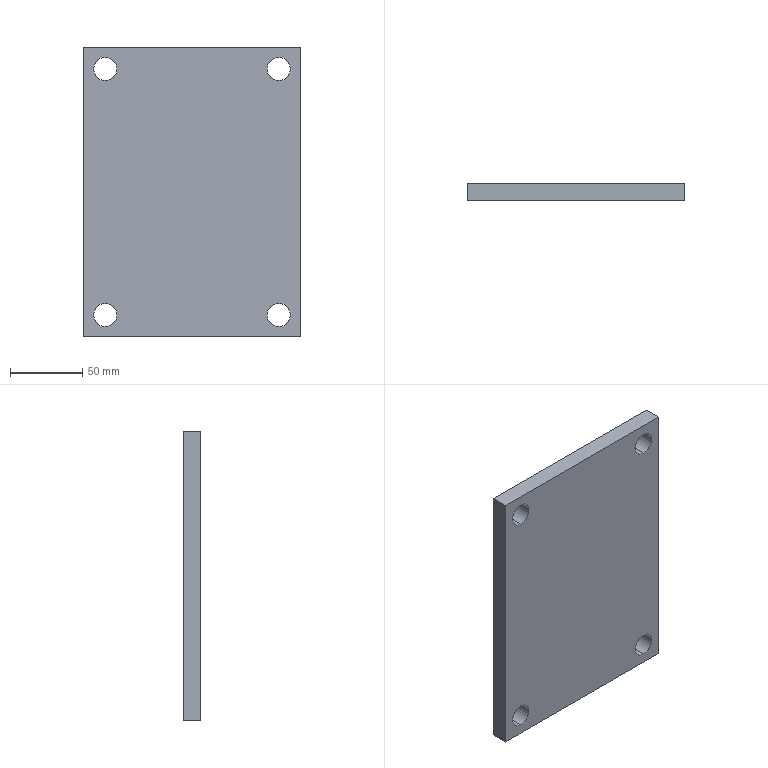Part | STEP file | E3-楼梯立柱Pad 1 | 1 solid | 14 faces | box 150 x 12 x 200 mm | volume 350349 mm3 | cylinder 8 | plane 6 | commonest cylinder face diameters 16 x8
STEP:
#1=CARTESIAN_POINT('',(0.,0.,0.));
#2=DIRECTION('',(0.,0.,1.));
#3=DIRECTION('',(1.,0.,0.));
#4=AXIS2_PLACEMENT_3D('',#1,#2,#3);
#5=CARTESIAN_POINT('',(60.,0.,-93.));
#6=VERTEX_POINT('',#5);
#7=CARTESIAN_POINT('',(60.,12.,-93.));
#8=VERTEX_POINT('',#7);
#9=CARTESIAN_POINT('',(60.,12.,-93.));
#10=DIRECTION('',(0.,1.,0.));
#11=VECTOR('',#10,1.);
#12=LINE('',#9,#11);
#13=CARTESIAN_POINT('',(60.,12.,-85.));
#14=DIRECTION('',(0.,1.,0.));
#15=DIRECTION('',(0.,0.,-1.));
#16=AXIS2_PLACEMENT_3D('',#13,#14,#15);
#17=CYLINDRICAL_SURFACE('',#16,8.);
#18=CARTESIAN_POINT('',(6.283,0.));
#19=DIRECTION('',(0.,1.));
#20=VECTOR('',#19,1.);
#21=LINE('',#18,#20);
#22=(GEOMETRIC_REPRESENTATION_CONTEXT(2)PARAMETRIC_REPRESENTATION_CONTEXT()REPRESENTATION_CONTEXT('',''));
#23=DEFINITIONAL_REPRESENTATION('',(#21),#22);
#24=PCURVE('',#17,#23);
#25=CARTESIAN_POINT('',(60.,12.,-85.));
#26=DIRECTION('',(0.,1.,0.));
#27=DIRECTION('',(0.,0.,-1.));
#28=AXIS2_PLACEMENT_3D('',#25,#26,#27);
#29=CYLINDRICAL_SURFACE('',#28,8.);
#30=CARTESIAN_POINT('',(0.,0.));
#31=DIRECTION('',(0.,1.));
#32=VECTOR('',#31,1.);
#33=LINE('',#30,#32);
#34=(GEOMETRIC_REPRESENTATION_CONTEXT(2)PARAMETRIC_REPRESENTATION_CONTEXT()REPRESENTATION_CONTEXT('',''));
#35=DEFINITIONAL_REPRESENTATION('',(#33),#34);
#36=PCURVE('',#29,#35);
#37=SURFACE_CURVE('',#12,(#24,#36),.PCURVE_S1.);
#38=EDGE_CURVE('',#6,#8,#37,.T.);
#39=ORIENTED_EDGE('',*,*,#38,.T.);
#40=CARTESIAN_POINT('',(60.,12.,-77.));
#41=VERTEX_POINT('',#40);
#42=CARTESIAN_POINT('',(60.,12.,-85.));
#43=DIRECTION('',(0.,-1.,0.));
#44=DIRECTION('',(0.,0.,-1.));
#45=AXIS2_PLACEMENT_3D('',#42,#43,#44);
#46=CIRCLE('',#45,8.);
#47=CARTESIAN_POINT('',(6.283,0.));
#48=DIRECTION('',(-1.,0.));
#49=VECTOR('',#48,1.);
#50=LINE('',#47,#49);
#51=(GEOMETRIC_REPRESENTATION_CONTEXT(2)PARAMETRIC_REPRESENTATION_CONTEXT()REPRESENTATION_CONTEXT('',''));
#52=DEFINITIONAL_REPRESENTATION('',(#50),#51);
#53=PCURVE('',#17,#52);
#54=CARTESIAN_POINT('',(0.,12.,0.));
#55=DIRECTION('',(0.,1.,0.));
#56=DIRECTION('',(0.,0.,-1.));
#57=AXIS2_PLACEMENT_3D('',#54,#55,#56);
#58=PLANE('',#57);
#59=CARTESIAN_POINT('',(93.,-60.));
#60=CARTESIAN_POINT('',(93.,-73.856));
#61=CARTESIAN_POINT('',(81.,-66.928));
#62=CARTESIAN_POINT('',(69.,-60.));
#63=CARTESIAN_POINT('',(81.,-53.072));
#64=CARTESIAN_POINT('',(93.,-46.144));
#65=CARTESIAN_POINT('',(93.,-60.));
#66=(BOUNDED_CURVE()B_SPLINE_CURVE(2,(#59,#60,#61,#62,#63,#64,#65),.UNSPECIFIED.,.T.,.F.)B_SPLINE_CURVE_WITH_KNOTS((1,2,2,2,2,1),(-2.094,0.,2.094,4.189,6.283,8.378),.UNSPECIFIED.)CURVE()GEOMETRIC_REPRESENTATION_ITEM()RATIONAL_B_SPLINE_CURVE((1.,0.5,1.,0.5,1.,0.5,1.))REPRESENTATION_ITEM(''));
#67=(GEOMETRIC_REPRESENTATION_CONTEXT(2)PARAMETRIC_REPRESENTATION_CONTEXT()REPRESENTATION_CONTEXT('',''));
#68=DEFINITIONAL_REPRESENTATION('',(#66),#67);
#69=PCURVE('',#58,#68);
#70=SURFACE_CURVE('',#46,(#53,#69),.PCURVE_S1.);
#71=EDGE_CURVE('',#8,#41,#70,.T.);
#72=ORIENTED_EDGE('',*,*,#71,.T.);
#73=CARTESIAN_POINT('',(60.,0.,-77.));
#74=VERTEX_POINT('',#73);
#75=CARTESIAN_POINT('',(60.,12.,-77.));
#76=DIRECTION('',(0.,1.,0.));
#77=VECTOR('',#76,1.);
#78=LINE('',#75,#77);
#79=CARTESIAN_POINT('',(3.142,0.));
#80=DIRECTION('',(0.,1.));
#81=VECTOR('',#80,1.);
#82=LINE('',#79,#81);
#83=(GEOMETRIC_REPRESENTATION_CONTEXT(2)PARAMETRIC_REPRESENTATION_CONTEXT()REPRESENTATION_CONTEXT('',''));
#84=DEFINITIONAL_REPRESENTATION('',(#82),#83);
#85=PCURVE('',#17,#84);
#86=CARTESIAN_POINT('',(3.142,0.));
#87=DIRECTION('',(0.,1.));
#88=VECTOR('',#87,1.);
#89=LINE('',#86,#88);
#90=(GEOMETRIC_REPRESENTATION_CONTEXT(2)PARAMETRIC_REPRESENTATION_CONTEXT()REPRESENTATION_CONTEXT('',''));
#91=DEFINITIONAL_REPRESENTATION('',(#89),#90);
#92=PCURVE('',#29,#91);
#93=SURFACE_CURVE('',#78,(#85,#92),.PCURVE_S1.);
#94=EDGE_CURVE('',#74,#41,#93,.T.);
#95=ORIENTED_EDGE('',*,*,#94,.F.);
#96=CARTESIAN_POINT('',(60.,0.,-85.));
#97=DIRECTION('',(0.,-1.,0.));
#98=DIRECTION('',(0.,0.,-1.));
#99=AXIS2_PLACEMENT_3D('',#96,#97,#98);
#100=CIRCLE('',#99,8.);
#101=CARTESIAN_POINT('',(6.283,-12.));
#102=DIRECTION('',(-1.,0.));
#103=VECTOR('',#102,1.);
#104=LINE('',#101,#103);
#105=(GEOMETRIC_REPRESENTATION_CONTEXT(2)PARAMETRIC_REPRESENTATION_CONTEXT()REPRESENTATION_CONTEXT('',''));
#106=DEFINITIONAL_REPRESENTATION('',(#104),#105);
#107=PCURVE('',#17,#106);
#108=CARTESIAN_POINT('',(0.,0.,0.));
#109=DIRECTION('',(0.,1.,0.));
#110=DIRECTION('',(0.,0.,-1.));
#111=AXIS2_PLACEMENT_3D('',#108,#109,#110);
#112=PLANE('',#111);
#113=CARTESIAN_POINT('',(93.,-60.));
#114=CARTESIAN_POINT('',(93.,-73.856));
#115=CARTESIAN_POINT('',(81.,-66.928));
#116=CARTESIAN_POINT('',(69.,-60.));
#117=CARTESIAN_POINT('',(81.,-53.072));
#118=CARTESIAN_POINT('',(93.,-46.144));
#119=CARTESIAN_POINT('',(93.,-60.));
#120=(BOUNDED_CURVE()B_SPLINE_CURVE(2,(#113,#114,#115,#116,#117,#118,#119),.UNSPECIFIED.,.T.,.F.)B_SPLINE_CURVE_WITH_KNOTS((1,2,2,2,2,1),(-2.094,0.,2.094,4.189,6.283,8.378),.UNSPECIFIED.)CURVE()GEOMETRIC_REPRESENTATION_ITEM()RATIONAL_B_SPLINE_CURVE((1.,0.5,1.,0.5,1.,0.5,1.))REPRESENTATION_ITEM(''));
#121=(GEOMETRIC_REPRESENTATION_CONTEXT(2)PARAMETRIC_REPRESENTATION_CONTEXT()REPRESENTATION_CONTEXT('',''));
#122=DEFINITIONAL_REPRESENTATION('',(#120),#121);
#123=PCURVE('',#112,#122);
#124=SURFACE_CURVE('',#100,(#107,#123),.PCURVE_S1.);
#125=EDGE_CURVE('',#6,#74,#124,.T.);
#126=ORIENTED_EDGE('',*,*,#125,.F.);
#127=EDGE_LOOP('',(#39,#72,#95,#126));
#128=FACE_BOUND('',#127,.F.);
#129=ADVANCED_FACE('',(#128),#17,.F.);
#130=CARTESIAN_POINT('',(-60.,0.,77.));
#131=VERTEX_POINT('',#130);
#132=CARTESIAN_POINT('',(-60.,12.,77.));
#133=VERTEX_POINT('',#132);
#134=CARTESIAN_POINT('',(-60.,12.,77.));
#135=DIRECTION('',(0.,1.,0.));
#136=VECTOR('',#135,1.);
#137=LINE('',#134,#136);
#138=CARTESIAN_POINT('',(-60.,12.,85.));
#139=DIRECTION('',(0.,1.,0.));
#140=DIRECTION('',(0.,0.,-1.));
#141=AXIS2_PLACEMENT_3D('',#138,#139,#140);
#142=CYLINDRICAL_SURFACE('',#141,8.);
#143=CARTESIAN_POINT('',(6.283,0.));
#144=DIRECTION('',(0.,1.));
#145=VECTOR('',#144,1.);
#146=LINE('',#143,#145);
#147=(GEOMETRIC_REPRESENTATION_CONTEXT(2)PARAMETRIC_REPRESENTATION_CONTEXT()REPRESENTATION_CONTEXT('',''));
#148=DEFINITIONAL_REPRESENTATION('',(#146),#147);
#149=PCURVE('',#142,#148);
#150=CARTESIAN_POINT('',(-60.,12.,85.));
#151=DIRECTION('',(0.,1.,0.));
#152=DIRECTION('',(0.,0.,-1.));
#153=AXIS2_PLACEMENT_3D('',#150,#151,#152);
#154=CYLINDRICAL_SURFACE('',#153,8.);
#155=CARTESIAN_POINT('',(0.,0.));
#156=DIRECTION('',(0.,1.));
#157=VECTOR('',#156,1.);
#158=LINE('',#155,#157);
#159=(GEOMETRIC_REPRESENTATION_CONTEXT(2)PARAMETRIC_REPRESENTATION_CONTEXT()REPRESENTATION_CONTEXT('',''));
#160=DEFINITIONAL_REPRESENTATION('',(#158),#159);
#161=PCURVE('',#154,#160);
#162=SURFACE_CURVE('',#137,(#149,#161),.PCURVE_S1.);
#163=EDGE_CURVE('',#131,#133,#162,.T.);
#164=ORIENTED_EDGE('',*,*,#163,.T.);
#165=CARTESIAN_POINT('',(-60.,12.,93.));
#166=VERTEX_POINT('',#165);
#167=CARTESIAN_POINT('',(-60.,12.,85.));
#168=DIRECTION('',(0.,-1.,0.));
#169=DIRECTION('',(0.,0.,-1.));
#170=AXIS2_PLACEMENT_3D('',#167,#168,#169);
#171=CIRCLE('',#170,8.);
#172=CARTESIAN_POINT('',(6.283,0.));
#173=DIRECTION('',(-1.,0.));
#174=VECTOR('',#173,1.);
#175=LINE('',#172,#174);
#176=(GEOMETRIC_REPRESENTATION_CONTEXT(2)PARAMETRIC_REPRESENTATION_CONTEXT()REPRESENTATION_CONTEXT('',''));
#177=DEFINITIONAL_REPRESENTATION('',(#175),#176);
#178=PCURVE('',#142,#177);
#179=CARTESIAN_POINT('',(-77.,60.));
#180=CARTESIAN_POINT('',(-77.,46.144));
#181=CARTESIAN_POINT('',(-89.,53.072));
#182=CARTESIAN_POINT('',(-101.,60.));
#183=CARTESIAN_POINT('',(-89.,66.928));
#184=CARTESIAN_POINT('',(-77.,73.856));
#185=CARTESIAN_POINT('',(-77.,60.));
#186=(BOUNDED_CURVE()B_SPLINE_CURVE(2,(#179,#180,#181,#182,#183,#184,#185),.UNSPECIFIED.,.T.,.F.)B_SPLINE_CURVE_WITH_KNOTS((1,2,2,2,2,1),(-2.094,0.,2.094,4.189,6.283,8.378),.UNSPECIFIED.)CURVE()GEOMETRIC_REPRESENTATION_ITEM()RATIONAL_B_SPLINE_CURVE((1.,0.5,1.,0.5,1.,0.5,1.))REPRESENTATION_ITEM(''));
#187=(GEOMETRIC_REPRESENTATION_CONTEXT(2)PARAMETRIC_REPRESENTATION_CONTEXT()REPRESENTATION_CONTEXT('',''));
#188=DEFINITIONAL_REPRESENTATION('',(#186),#187);
#189=PCURVE('',#58,#188);
#190=SURFACE_CURVE('',#171,(#178,#189),.PCURVE_S1.);
#191=EDGE_CURVE('',#133,#166,#190,.T.);
#192=ORIENTED_EDGE('',*,*,#191,.T.);
#193=CARTESIAN_POINT('',(-60.,0.,93.));
#194=VERTEX_POINT('',#193);
#195=CARTESIAN_POINT('',(-60.,12.,93.));
#196=DIRECTION('',(0.,1.,0.));
#197=VECTOR('',#196,1.);
#198=LINE('',#195,#197);
#199=CARTESIAN_POINT('',(3.142,0.));
#200=DIRECTION('',(0.,1.));
#201=VECTOR('',#200,1.);
#202=LINE('',#199,#201);
#203=(GEOMETRIC_REPRESENTATION_CONTEXT(2)PARAMETRIC_REPRESENTATION_CONTEXT()REPRESENTATION_CONTEXT('',''));
#204=DEFINITIONAL_REPRESENTATION('',(#202),#203);
#205=PCURVE('',#142,#204);
#206=CARTESIAN_POINT('',(3.142,0.));
#207=DIRECTION('',(0.,1.));
#208=VECTOR('',#207,1.);
#209=LINE('',#206,#208);
#210=(GEOMETRIC_REPRESENTATION_CONTEXT(2)PARAMETRIC_REPRESENTATION_CONTEXT()REPRESENTATION_CONTEXT('',''));
#211=DEFINITIONAL_REPRESENTATION('',(#209),#210);
#212=PCURVE('',#154,#211);
#213=SURFACE_CURVE('',#198,(#205,#212),.PCURVE_S1.);
#214=EDGE_CURVE('',#194,#166,#213,.T.);
#215=ORIENTED_EDGE('',*,*,#214,.F.);
#216=CARTESIAN_POINT('',(-60.,0.,85.));
#217=DIRECTION('',(0.,-1.,0.));
#218=DIRECTION('',(0.,0.,-1.));
#219=AXIS2_PLACEMENT_3D('',#216,#217,#218);
#220=CIRCLE('',#219,8.);
#221=CARTESIAN_POINT('',(6.283,-12.));
#222=DIRECTION('',(-1.,0.));
#223=VECTOR('',#222,1.);
#224=LINE('',#221,#223);
#225=(GEOMETRIC_REPRESENTATION_CONTEXT(2)PARAMETRIC_REPRESENTATION_CONTEXT()REPRESENTATION_CONTEXT('',''));
#226=DEFINITIONAL_REPRESENTATION('',(#224),#225);
#227=PCURVE('',#142,#226);
#228=CARTESIAN_POINT('',(-77.,60.));
#229=CARTESIAN_POINT('',(-77.,46.144));
#230=CARTESIAN_POINT('',(-89.,53.072));
#231=CARTESIAN_POINT('',(-101.,60.));
#232=CARTESIAN_POINT('',(-89.,66.928));
#233=CARTESIAN_POINT('',(-77.,73.856));
#234=CARTESIAN_POINT('',(-77.,60.));
#235=(BOUNDED_CURVE()B_SPLINE_CURVE(2,(#228,#229,#230,#231,#232,#233,#234),.UNSPECIFIED.,.T.,.F.)B_SPLINE_CURVE_WITH_KNOTS((1,2,2,2,2,1),(-2.094,0.,2.094,4.189,6.283,8.378),.UNSPECIFIED.)CURVE()GEOMETRIC_REPRESENTATION_ITEM()RATIONAL_B_SPLINE_CURVE((1.,0.5,1.,0.5,1.,0.5,1.))REPRESENTATION_ITEM(''));
#236=(GEOMETRIC_REPRESENTATION_CONTEXT(2)PARAMETRIC_REPRESENTATION_CONTEXT()REPRESENTATION_CONTEXT('',''));
#237=DEFINITIONAL_REPRESENTATION('',(#235),#236);
#238=PCURVE('',#112,#237);
#239=SURFACE_CURVE('',#220,(#227,#238),.PCURVE_S1.);
#240=EDGE_CURVE('',#131,#194,#239,.T.);
#241=ORIENTED_EDGE('',*,*,#240,.F.);
#242=EDGE_LOOP('',(#164,#192,#215,#241));
#243=FACE_BOUND('',#242,.F.);
#244=ADVANCED_FACE('',(#243),#142,.F.);
#245=CARTESIAN_POINT('',(-60.,0.,-93.));
#246=VERTEX_POINT('',#245);
#247=CARTESIAN_POINT('',(-60.,12.,-93.));
#248=VERTEX_POINT('',#247);
#249=CARTESIAN_POINT('',(-60.,12.,-93.));
#250=DIRECTION('',(0.,1.,0.));
#251=VECTOR('',#250,1.);
#252=LINE('',#249,#251);
#253=CARTESIAN_POINT('',(-60.,12.,-85.));
#254=DIRECTION('',(0.,1.,0.));
#255=DIRECTION('',(0.,0.,-1.));
#256=AXIS2_PLACEMENT_3D('',#253,#254,#255);
#257=CYLINDRICAL_SURFACE('',#256,8.);
#258=CARTESIAN_POINT('',(6.283,0.));
#259=DIRECTION('',(0.,1.));
#260=VECTOR('',#259,1.);
#261=LINE('',#258,#260);
#262=(GEOMETRIC_REPRESENTATION_CONTEXT(2)PARAMETRIC_REPRESENTATION_CONTEXT()REPRESENTATION_CONTEXT('',''));
#263=DEFINITIONAL_REPRESENTATION('',(#261),#262);
#264=PCURVE('',#257,#263);
#265=CARTESIAN_POINT('',(-60.,12.,-85.));
#266=DIRECTION('',(0.,1.,0.));
#267=DIRECTION('',(0.,0.,-1.));
#268=AXIS2_PLACEMENT_3D('',#265,#266,#267);
#269=CYLINDRICAL_SURFACE('',#268,8.);
#270=CARTESIAN_POINT('',(0.,0.));
#271=DIRECTION('',(0.,1.));
#272=VECTOR('',#271,1.);
#273=LINE('',#270,#272);
#274=(GEOMETRIC_REPRESENTATION_CONTEXT(2)PARAMETRIC_REPRESENTATION_CONTEXT()REPRESENTATION_CONTEXT('',''));
#275=DEFINITIONAL_REPRESENTATION('',(#273),#274);
#276=PCURVE('',#269,#275);
#277=SURFACE_CURVE('',#252,(#264,#276),.PCURVE_S1.);
#278=EDGE_CURVE('',#246,#248,#277,.T.);
#279=ORIENTED_EDGE('',*,*,#278,.T.);
#280=CARTESIAN_POINT('',(-60.,12.,-77.));
#281=VERTEX_POINT('',#280);
#282=CARTESIAN_POINT('',(-60.,12.,-85.));
#283=DIRECTION('',(0.,-1.,0.));
#284=DIRECTION('',(0.,0.,-1.));
#285=AXIS2_PLACEMENT_3D('',#282,#283,#284);
#286=CIRCLE('',#285,8.);
#287=CARTESIAN_POINT('',(6.283,0.));
#288=DIRECTION('',(-1.,0.));
#289=VECTOR('',#288,1.);
#290=LINE('',#287,#289);
#291=(GEOMETRIC_REPRESENTATION_CONTEXT(2)PARAMETRIC_REPRESENTATION_CONTEXT()REPRESENTATION_CONTEXT('',''));
#292=DEFINITIONAL_REPRESENTATION('',(#290),#291);
#293=PCURVE('',#257,#292);
#294=CARTESIAN_POINT('',(93.,60.));
#295=CARTESIAN_POINT('',(93.,46.144));
#296=CARTESIAN_POINT('',(81.,53.072));
#297=CARTESIAN_POINT('',(69.,60.));
#298=CARTESIAN_POINT('',(81.,66.928));
#299=CARTESIAN_POINT('',(93.,73.856));
#300=CARTESIAN_POINT('',(93.,60.));
#301=(BOUNDED_CURVE()B_SPLINE_CURVE(2,(#294,#295,#296,#297,#298,#299,#300),.UNSPECIFIED.,.T.,.F.)B_SPLINE_CURVE_WITH_KNOTS((1,2,2,2,2,1),(-2.094,0.,2.094,4.189,6.283,8.378),.UNSPECIFIED.)CURVE()GEOMETRIC_REPRESENTATION_ITEM()RATIONAL_B_SPLINE_CURVE((1.,0.5,1.,0.5,1.,0.5,1.))REPRESENTATION_ITEM(''));
#302=(GEOMETRIC_REPRESENTATION_CONTEXT(2)PARAMETRIC_REPRESENTATION_CONTEXT()REPRESENTATION_CONTEXT('',''));
#303=DEFINITIONAL_REPRESENTATION('',(#301),#302);
#304=PCURVE('',#58,#303);
#305=SURFACE_CURVE('',#286,(#293,#304),.PCURVE_S1.);
#306=EDGE_CURVE('',#248,#281,#305,.T.);
#307=ORIENTED_EDGE('',*,*,#306,.T.);
#308=CARTESIAN_POINT('',(-60.,0.,-77.));
#309=VERTEX_POINT('',#308);
#310=CARTESIAN_POINT('',(-60.,12.,-77.));
#311=DIRECTION('',(0.,1.,0.));
#312=VECTOR('',#311,1.);
#313=LINE('',#310,#312);
#314=CARTESIAN_POINT('',(3.142,0.));
#315=DIRECTION('',(0.,1.));
#316=VECTOR('',#315,1.);
#317=LINE('',#314,#316);
#318=(GEOMETRIC_REPRESENTATION_CONTEXT(2)PARAMETRIC_REPRESENTATION_CONTEXT()REPRESENTATION_CONTEXT('',''));
#319=DEFINITIONAL_REPRESENTATION('',(#317),#318);
#320=PCURVE('',#257,#319);
#321=CARTESIAN_POINT('',(3.142,0.));
#322=DIRECTION('',(0.,1.));
#323=VECTOR('',#322,1.);
#324=LINE('',#321,#323);
#325=(GEOMETRIC_REPRESENTATION_CONTEXT(2)PARAMETRIC_REPRESENTATION_CONTEXT()REPRESENTATION_CONTEXT('',''));
#326=DEFINITIONAL_REPRESENTATION('',(#324),#325);
#327=PCURVE('',#269,#326);
#328=SURFACE_CURVE('',#313,(#320,#327),.PCURVE_S1.);
#329=EDGE_CURVE('',#309,#281,#328,.T.);
#330=ORIENTED_EDGE('',*,*,#329,.F.);
#331=CARTESIAN_POINT('',(-60.,0.,-85.));
#332=DIRECTION('',(0.,-1.,0.));
#333=DIRECTION('',(0.,0.,-1.));
#334=AXIS2_PLACEMENT_3D('',#331,#332,#333);
#335=CIRCLE('',#334,8.);
#336=CARTESIAN_POINT('',(6.283,-12.));
#337=DIRECTION('',(-1.,0.));
#338=VECTOR('',#337,1.);
#339=LINE('',#336,#338);
#340=(GEOMETRIC_REPRESENTATION_CONTEXT(2)PARAMETRIC_REPRESENTATION_CONTEXT()REPRESENTATION_CONTEXT('',''));
#341=DEFINITIONAL_REPRESENTATION('',(#339),#340);
#342=PCURVE('',#257,#341);
#343=CARTESIAN_POINT('',(93.,60.));
#344=CARTESIAN_POINT('',(93.,46.144));
#345=CARTESIAN_POINT('',(81.,53.072));
#346=CARTESIAN_POINT('',(69.,60.));
#347=CARTESIAN_POINT('',(81.,66.928));
#348=CARTESIAN_POINT('',(93.,73.856));
#349=CARTESIAN_POINT('',(93.,60.));
#350=(BOUNDED_CURVE()B_SPLINE_CURVE(2,(#343,#344,#345,#346,#347,#348,#349),.UNSPECIFIED.,.T.,.F.)B_SPLINE_CURVE_WITH_KNOTS((1,2,2,2,2,1),(-2.094,0.,2.094,4.189,6.283,8.378),.UNSPECIFIED.)CURVE()GEOMETRIC_REPRESENTATION_ITEM()RATIONAL_B_SPLINE_CURVE((1.,0.5,1.,0.5,1.,0.5,1.))REPRESENTATION_ITEM(''));
#351=(GEOMETRIC_REPRESENTATION_CONTEXT(2)PARAMETRIC_REPRESENTATION_CONTEXT()REPRESENTATION_CONTEXT('',''));
#352=DEFINITIONAL_REPRESENTATION('',(#350),#351);
#353=PCURVE('',#112,#352);
#354=SURFACE_CURVE('',#335,(#342,#353),.PCURVE_S1.);
#355=EDGE_CURVE('',#246,#309,#354,.T.);
#356=ORIENTED_EDGE('',*,*,#355,.F.);
#357=EDGE_LOOP('',(#279,#307,#330,#356));
#358=FACE_BOUND('',#357,.F.);
#359=ADVANCED_FACE('',(#358),#257,.F.);
#360=CARTESIAN_POINT('',(60.,0.,77.));
#361=VERTEX_POINT('',#360);
#362=CARTESIAN_POINT('',(60.,12.,77.));
#363=VERTEX_POINT('',#362);
#364=CARTESIAN_POINT('',(60.,12.,77.));
#365=DIRECTION('',(0.,1.,0.));
#366=VECTOR('',#365,1.);
#367=LINE('',#364,#366);
#368=CARTESIAN_POINT('',(60.,12.,85.));
#369=DIRECTION('',(0.,1.,0.));
#370=DIRECTION('',(0.,0.,-1.));
#371=AXIS2_PLACEMENT_3D('',#368,#369,#370);
#372=CYLINDRICAL_SURFACE('',#371,8.);
#373=CARTESIAN_POINT('',(6.283,0.));
#374=DIRECTION('',(0.,1.));
#375=VECTOR('',#374,1.);
#376=LINE('',#373,#375);
#377=(GEOMETRIC_REPRESENTATION_CONTEXT(2)PARAMETRIC_REPRESENTATION_CONTEXT()REPRESENTATION_CONTEXT('',''));
#378=DEFINITIONAL_REPRESENTATION('',(#376),#377);
#379=PCURVE('',#372,#378);
#380=CARTESIAN_POINT('',(60.,12.,85.));
#381=DIRECTION('',(0.,1.,0.));
#382=DIRECTION('',(0.,0.,-1.));
#383=AXIS2_PLACEMENT_3D('',#380,#381,#382);
#384=CYLINDRICAL_SURFACE('',#383,8.);
#385=CARTESIAN_POINT('',(0.,0.));
#386=DIRECTION('',(0.,1.));
#387=VECTOR('',#386,1.);
#388=LINE('',#385,#387);
#389=(GEOMETRIC_REPRESENTATION_CONTEXT(2)PARAMETRIC_REPRESENTATION_CONTEXT()REPRESENTATION_CONTEXT('',''));
#390=DEFINITIONAL_REPRESENTATION('',(#388),#389);
#391=PCURVE('',#384,#390);
#392=SURFACE_CURVE('',#367,(#379,#391),.PCURVE_S1.);
#393=EDGE_CURVE('',#361,#363,#392,.T.);
#394=ORIENTED_EDGE('',*,*,#393,.T.);
#395=CARTESIAN_POINT('',(60.,12.,93.));
#396=VERTEX_POINT('',#395);
#397=CARTESIAN_POINT('',(60.,12.,85.));
#398=DIRECTION('',(0.,-1.,0.));
#399=DIRECTION('',(0.,0.,-1.));
#400=AXIS2_PLACEMENT_3D('',#397,#398,#399);
#401=CIRCLE('',#400,8.);
#402=CARTESIAN_POINT('',(6.283,0.));
#403=DIRECTION('',(-1.,0.));
#404=VECTOR('',#403,1.);
#405=LINE('',#402,#404);
#406=(GEOMETRIC_REPRESENTATION_CONTEXT(2)PARAMETRIC_REPRESENTATION_CONTEXT()REPRESENTATION_CONTEXT('',''));
#407=DEFINITIONAL_REPRESENTATION('',(#405),#406);
#408=PCURVE('',#372,#407);
#409=CARTESIAN_POINT('',(-77.,-60.));
#410=CARTESIAN_POINT('',(-77.,-73.856));
#411=CARTESIAN_POINT('',(-89.,-66.928));
#412=CARTESIAN_POINT('',(-101.,-60.));
#413=CARTESIAN_POINT('',(-89.,-53.072));
#414=CARTESIAN_POINT('',(-77.,-46.144));
#415=CARTESIAN_POINT('',(-77.,-60.));
#416=(BOUNDED_CURVE()B_SPLINE_CURVE(2,(#409,#410,#411,#412,#413,#414,#415),.UNSPECIFIED.,.T.,.F.)B_SPLINE_CURVE_WITH_KNOTS((1,2,2,2,2,1),(-2.094,0.,2.094,4.189,6.283,8.378),.UNSPECIFIED.)CURVE()GEOMETRIC_REPRESENTATION_ITEM()RATIONAL_B_SPLINE_CURVE((1.,0.5,1.,0.5,1.,0.5,1.))REPRESENTATION_ITEM(''));
#417=(GEOMETRIC_REPRESENTATION_CONTEXT(2)PARAMETRIC_REPRESENTATION_CONTEXT()REPRESENTATION_CONTEXT('',''));
#418=DEFINITIONAL_REPRESENTATION('',(#416),#417);
#419=PCURVE('',#58,#418);
#420=SURFACE_CURVE('',#401,(#408,#419),.PCURVE_S1.);
#421=EDGE_CURVE('',#363,#396,#420,.T.);
#422=ORIENTED_EDGE('',*,*,#421,.T.);
#423=CARTESIAN_POINT('',(60.,0.,93.));
#424=VERTEX_POINT('',#423);
#425=CARTESIAN_POINT('',(60.,12.,93.));
#426=DIRECTION('',(0.,1.,0.));
#427=VECTOR('',#426,1.);
#428=LINE('',#425,#427);
#429=CARTESIAN_POINT('',(3.142,0.));
#430=DIRECTION('',(0.,1.));
#431=VECTOR('',#430,1.);
#432=LINE('',#429,#431);
#433=(GEOMETRIC_REPRESENTATION_CONTEXT(2)PARAMETRIC_REPRESENTATION_CONTEXT()REPRESENTATION_CONTEXT('',''));
#434=DEFINITIONAL_REPRESENTATION('',(#432),#433);
#435=PCURVE('',#372,#434);
#436=CARTESIAN_POINT('',(3.142,0.));
#437=DIRECTION('',(0.,1.));
#438=VECTOR('',#437,1.);
#439=LINE('',#436,#438);
#440=(GEOMETRIC_REPRESENTATION_CONTEXT(2)PARAMETRIC_REPRESENTATION_CONTEXT()REPRESENTATION_CONTEXT('',''));
#441=DEFINITIONAL_REPRESENTATION('',(#439),#440);
#442=PCURVE('',#384,#441);
#443=SURFACE_CURVE('',#428,(#435,#442),.PCURVE_S1.);
#444=EDGE_CURVE('',#424,#396,#443,.T.);
#445=ORIENTED_EDGE('',*,*,#444,.F.);
#446=CARTESIAN_POINT('',(60.,0.,85.));
#447=DIRECTION('',(0.,-1.,0.));
#448=DIRECTION('',(0.,0.,-1.));
#449=AXIS2_PLACEMENT_3D('',#446,#447,#448);
#450=CIRCLE('',#449,8.);
#451=CARTESIAN_POINT('',(6.283,-12.));
#452=DIRECTION('',(-1.,0.));
#453=VECTOR('',#452,1.);
#454=LINE('',#451,#453);
#455=(GEOMETRIC_REPRESENTATION_CONTEXT(2)PARAMETRIC_REPRESENTATION_CONTEXT()REPRESENTATION_CONTEXT('',''));
#456=DEFINITIONAL_REPRESENTATION('',(#454),#455);
#457=PCURVE('',#372,#456);
#458=CARTESIAN_POINT('',(-77.,-60.));
#459=CARTESIAN_POINT('',(-77.,-73.856));
#460=CARTESIAN_POINT('',(-89.,-66.928));
#461=CARTESIAN_POINT('',(-101.,-60.));
#462=CARTESIAN_POINT('',(-89.,-53.072));
#463=CARTESIAN_POINT('',(-77.,-46.144));
#464=CARTESIAN_POINT('',(-77.,-60.));
#465=(BOUNDED_CURVE()B_SPLINE_CURVE(2,(#458,#459,#460,#461,#462,#463,#464),.UNSPECIFIED.,.T.,.F.)B_SPLINE_CURVE_WITH_KNOTS((1,2,2,2,2,1),(-2.094,0.,2.094,4.189,6.283,8.378),.UNSPECIFIED.)CURVE()GEOMETRIC_REPRESENTATION_ITEM()RATIONAL_B_SPLINE_CURVE((1.,0.5,1.,0.5,1.,0.5,1.))REPRESENTATION_ITEM(''));
#466=(GEOMETRIC_REPRESENTATION_CONTEXT(2)PARAMETRIC_REPRESENTATION_CONTEXT()REPRESENTATION_CONTEXT('',''));
#467=DEFINITIONAL_REPRESENTATION('',(#465),#466);
#468=PCURVE('',#112,#467);
#469=SURFACE_CURVE('',#450,(#457,#468),.PCURVE_S1.);
#470=EDGE_CURVE('',#361,#424,#469,.T.);
#471=ORIENTED_EDGE('',*,*,#470,.F.);
#472=EDGE_LOOP('',(#394,#422,#445,#471));
#473=FACE_BOUND('',#472,.F.);
#474=ADVANCED_FACE('',(#473),#372,.F.);
#475=CARTESIAN_POINT('',(75.,0.,-100.));
#476=VERTEX_POINT('',#475);
#477=CARTESIAN_POINT('',(75.,0.,100.));
#478=VERTEX_POINT('',#477);
#479=CARTESIAN_POINT('',(75.,0.,100.));
#480=DIRECTION('',(0.,0.,1.));
#481=VECTOR('',#480,1.);
#482=LINE('',#479,#481);
#483=CARTESIAN_POINT('',(75.,12.,100.));
#484=DIRECTION('',(-1.,0.,0.));
#485=DIRECTION('',(0.,0.,-1.));
#486=AXIS2_PLACEMENT_3D('',#483,#484,#485);
#487=PLANE('',#486);
#488=CARTESIAN_POINT('',(0.,12.));
#489=DIRECTION('',(-1.,0.));
#490=VECTOR('',#489,1.);
#491=LINE('',#488,#490);
#492=(GEOMETRIC_REPRESENTATION_CONTEXT(2)PARAMETRIC_REPRESENTATION_CONTEXT()REPRESENTATION_CONTEXT('',''));
#493=DEFINITIONAL_REPRESENTATION('',(#491),#492);
#494=PCURVE('',#487,#493);
#495=CARTESIAN_POINT('',(-100.,-75.));
#496=DIRECTION('',(-1.,0.));
#497=VECTOR('',#496,1.);
#498=LINE('',#495,#497);
#499=(GEOMETRIC_REPRESENTATION_CONTEXT(2)PARAMETRIC_REPRESENTATION_CONTEXT()REPRESENTATION_CONTEXT('',''));
#500=DEFINITIONAL_REPRESENTATION('',(#498),#499);
#501=PCURVE('',#112,#500);
#502=SURFACE_CURVE('',#482,(#494,#501),.PCURVE_S1.);
#503=EDGE_CURVE('',#476,#478,#502,.T.);
#504=ORIENTED_EDGE('',*,*,#503,.F.);
#505=CARTESIAN_POINT('',(75.,12.,-100.));
#506=VERTEX_POINT('',#505);
#507=CARTESIAN_POINT('',(75.,12.,-100.));
#508=DIRECTION('',(0.,-1.,0.));
#509=VECTOR('',#508,1.);
#510=LINE('',#507,#509);
#511=CARTESIAN_POINT('',(200.,0.));
#512=DIRECTION('',(0.,1.));
#513=VECTOR('',#512,1.);
#514=LINE('',#511,#513);
#515=(GEOMETRIC_REPRESENTATION_CONTEXT(2)PARAMETRIC_REPRESENTATION_CONTEXT()REPRESENTATION_CONTEXT('',''));
#516=DEFINITIONAL_REPRESENTATION('',(#514),#515);
#517=PCURVE('',#487,#516);
#518=CARTESIAN_POINT('',(-75.,12.,-100.));
#519=DIRECTION('',(0.,0.,1.));
#520=DIRECTION('',(-1.,0.,0.));
#521=AXIS2_PLACEMENT_3D('',#518,#519,#520);
#522=PLANE('',#521);
#523=CARTESIAN_POINT('',(-150.,0.));
#524=DIRECTION('',(0.,1.));
#525=VECTOR('',#524,1.);
#526=LINE('',#523,#525);
#527=(GEOMETRIC_REPRESENTATION_CONTEXT(2)PARAMETRIC_REPRESENTATION_CONTEXT()REPRESENTATION_CONTEXT('',''));
#528=DEFINITIONAL_REPRESENTATION('',(#526),#527);
#529=PCURVE('',#522,#528);
#530=SURFACE_CURVE('',#510,(#517,#529),.PCURVE_S1.);
#531=EDGE_CURVE('',#506,#476,#530,.T.);
#532=ORIENTED_EDGE('',*,*,#531,.F.);
#533=CARTESIAN_POINT('',(75.,12.,100.));
#534=VERTEX_POINT('',#533);
#535=CARTESIAN_POINT('',(75.,12.,100.));
#536=DIRECTION('',(0.,0.,1.));
#537=VECTOR('',#536,1.);
#538=LINE('',#535,#537);
#539=CARTESIAN_POINT('',(0.,0.));
#540=DIRECTION('',(-1.,0.));
#541=VECTOR('',#540,1.);
#542=LINE('',#539,#541);
#543=(GEOMETRIC_REPRESENTATION_CONTEXT(2)PARAMETRIC_REPRESENTATION_CONTEXT()REPRESENTATION_CONTEXT('',''));
#544=DEFINITIONAL_REPRESENTATION('',(#542),#543);
#545=PCURVE('',#487,#544);
#546=CARTESIAN_POINT('',(-100.,-75.));
#547=DIRECTION('',(-1.,0.));
#548=VECTOR('',#547,1.);
#549=LINE('',#546,#548);
#550=(GEOMETRIC_REPRESENTATION_CONTEXT(2)PARAMETRIC_REPRESENTATION_CONTEXT()REPRESENTATION_CONTEXT('',''));
#551=DEFINITIONAL_REPRESENTATION('',(#549),#550);
#552=PCURVE('',#58,#551);
#553=SURFACE_CURVE('',#538,(#545,#552),.PCURVE_S1.);
#554=EDGE_CURVE('',#506,#534,#553,.T.);
#555=ORIENTED_EDGE('',*,*,#554,.T.);
#556=CARTESIAN_POINT('',(75.,12.,100.));
#557=DIRECTION('',(0.,-1.,0.));
#558=VECTOR('',#557,1.);
#559=LINE('',#556,#558);
#560=CARTESIAN_POINT('',(0.,0.));
#561=DIRECTION('',(0.,1.));
#562=VECTOR('',#561,1.);
#563=LINE('',#560,#562);
#564=(GEOMETRIC_REPRESENTATION_CONTEXT(2)PARAMETRIC_REPRESENTATION_CONTEXT()REPRESENTATION_CONTEXT('',''));
#565=DEFINITIONAL_REPRESENTATION('',(#563),#564);
#566=PCURVE('',#487,#565);
#567=CARTESIAN_POINT('',(-75.,12.,100.));
#568=DIRECTION('',(0.,0.,-1.));
#569=DIRECTION('',(1.,0.,0.));
#570=AXIS2_PLACEMENT_3D('',#567,#568,#569);
#571=PLANE('',#570);
#572=CARTESIAN_POINT('',(150.,0.));
#573=DIRECTION('',(0.,1.));
#574=VECTOR('',#573,1.);
#575=LINE('',#572,#574);
#576=(GEOMETRIC_REPRESENTATION_CONTEXT(2)PARAMETRIC_REPRESENTATION_CONTEXT()REPRESENTATION_CONTEXT('',''));
#577=DEFINITIONAL_REPRESENTATION('',(#575),#576);
#578=PCURVE('',#571,#577);
#579=SURFACE_CURVE('',#559,(#566,#578),.PCURVE_S1.);
#580=EDGE_CURVE('',#534,#478,#579,.T.);
#581=ORIENTED_EDGE('',*,*,#580,.T.);
#582=EDGE_LOOP('',(#504,#532,#555,#581));
#583=FACE_BOUND('',#582,.T.);
#584=ADVANCED_FACE('',(#583),#487,.F.);
#585=CARTESIAN_POINT('',(-75.,0.,100.));
#586=VERTEX_POINT('',#585);
#587=CARTESIAN_POINT('',(-75.,0.,100.));
#588=DIRECTION('',(-1.,0.,0.));
#589=VECTOR('',#588,1.);
#590=LINE('',#587,#589);
#591=CARTESIAN_POINT('',(0.,12.));
#592=DIRECTION('',(-1.,0.));
#593=VECTOR('',#592,1.);
#594=LINE('',#591,#593);
#595=(GEOMETRIC_REPRESENTATION_CONTEXT(2)PARAMETRIC_REPRESENTATION_CONTEXT()REPRESENTATION_CONTEXT('',''));
#596=DEFINITIONAL_REPRESENTATION('',(#594),#595);
#597=PCURVE('',#571,#596);
#598=CARTESIAN_POINT('',(-100.,75.));
#599=DIRECTION('',(0.,1.));
#600=VECTOR('',#599,1.);
#601=LINE('',#598,#600);
#602=(GEOMETRIC_REPRESENTATION_CONTEXT(2)PARAMETRIC_REPRESENTATION_CONTEXT()REPRESENTATION_CONTEXT('',''));
#603=DEFINITIONAL_REPRESENTATION('',(#601),#602);
#604=PCURVE('',#112,#603);
#605=SURFACE_CURVE('',#590,(#597,#604),.PCURVE_S1.);
#606=EDGE_CURVE('',#478,#586,#605,.T.);
#607=ORIENTED_EDGE('',*,*,#606,.F.);
#608=ORIENTED_EDGE('',*,*,#580,.F.);
#609=CARTESIAN_POINT('',(-75.,12.,100.));
#610=VERTEX_POINT('',#609);
#611=CARTESIAN_POINT('',(-75.,12.,100.));
#612=DIRECTION('',(-1.,0.,0.));
#613=VECTOR('',#612,1.);
#614=LINE('',#611,#613);
#615=CARTESIAN_POINT('',(0.,0.));
#616=DIRECTION('',(-1.,0.));
#617=VECTOR('',#616,1.);
#618=LINE('',#615,#617);
#619=(GEOMETRIC_REPRESENTATION_CONTEXT(2)PARAMETRIC_REPRESENTATION_CONTEXT()REPRESENTATION_CONTEXT('',''));
#620=DEFINITIONAL_REPRESENTATION('',(#618),#619);
#621=PCURVE('',#571,#620);
#622=CARTESIAN_POINT('',(-100.,75.));
#623=DIRECTION('',(0.,1.));
#624=VECTOR('',#623,1.);
#625=LINE('',#622,#624);
#626=(GEOMETRIC_REPRESENTATION_CONTEXT(2)PARAMETRIC_REPRESENTATION_CONTEXT()REPRESENTATION_CONTEXT('',''));
#627=DEFINITIONAL_REPRESENTATION('',(#625),#626);
#628=PCURVE('',#58,#627);
#629=SURFACE_CURVE('',#614,(#621,#628),.PCURVE_S1.);
#630=EDGE_CURVE('',#534,#610,#629,.T.);
#631=ORIENTED_EDGE('',*,*,#630,.T.);
#632=CARTESIAN_POINT('',(-75.,12.,100.));
#633=DIRECTION('',(0.,-1.,0.));
#634=VECTOR('',#633,1.);
#635=LINE('',#632,#634);
#636=CARTESIAN_POINT('',(0.,0.));
#637=DIRECTION('',(0.,1.));
#638=VECTOR('',#637,1.);
#639=LINE('',#636,#638);
#640=(GEOMETRIC_REPRESENTATION_CONTEXT(2)PARAMETRIC_REPRESENTATION_CONTEXT()REPRESENTATION_CONTEXT('',''));
#641=DEFINITIONAL_REPRESENTATION('',(#639),#640);
#642=PCURVE('',#571,#641);
#643=CARTESIAN_POINT('',(-75.,12.,100.));
#644=DIRECTION('',(1.,0.,0.));
#645=DIRECTION('',(0.,0.,1.));
#646=AXIS2_PLACEMENT_3D('',#643,#644,#645);
#647=PLANE('',#646);
#648=CARTESIAN_POINT('',(0.,0.));
#649=DIRECTION('',(0.,1.));
#650=VECTOR('',#649,1.);
#651=LINE('',#648,#650);
#652=(GEOMETRIC_REPRESENTATION_CONTEXT(2)PARAMETRIC_REPRESENTATION_CONTEXT()REPRESENTATION_CONTEXT('',''));
#653=DEFINITIONAL_REPRESENTATION('',(#651),#652);
#654=PCURVE('',#647,#653);
#655=SURFACE_CURVE('',#635,(#642,#654),.PCURVE_S1.);
#656=EDGE_CURVE('',#610,#586,#655,.T.);
#657=ORIENTED_EDGE('',*,*,#656,.T.);
#658=EDGE_LOOP('',(#607,#608,#631,#657));
#659=FACE_BOUND('',#658,.T.);
#660=ADVANCED_FACE('',(#659),#571,.F.);
#661=CARTESIAN_POINT('',(-75.,0.,-100.));
#662=VERTEX_POINT('',#661);
#663=CARTESIAN_POINT('',(-75.,0.,100.));
#664=DIRECTION('',(0.,0.,-1.));
#665=VECTOR('',#664,1.);
#666=LINE('',#663,#665);
#667=CARTESIAN_POINT('',(0.,12.));
#668=DIRECTION('',(-1.,0.));
#669=VECTOR('',#668,1.);
#670=LINE('',#667,#669);
#671=(GEOMETRIC_REPRESENTATION_CONTEXT(2)PARAMETRIC_REPRESENTATION_CONTEXT()REPRESENTATION_CONTEXT('',''));
#672=DEFINITIONAL_REPRESENTATION('',(#670),#671);
#673=PCURVE('',#647,#672);
#674=CARTESIAN_POINT('',(-100.,75.));
#675=DIRECTION('',(1.,0.));
#676=VECTOR('',#675,1.);
#677=LINE('',#674,#676);
#678=(GEOMETRIC_REPRESENTATION_CONTEXT(2)PARAMETRIC_REPRESENTATION_CONTEXT()REPRESENTATION_CONTEXT('',''));
#679=DEFINITIONAL_REPRESENTATION('',(#677),#678);
#680=PCURVE('',#112,#679);
#681=SURFACE_CURVE('',#666,(#673,#680),.PCURVE_S1.);
#682=EDGE_CURVE('',#586,#662,#681,.T.);
#683=ORIENTED_EDGE('',*,*,#682,.F.);
#684=ORIENTED_EDGE('',*,*,#656,.F.);
#685=CARTESIAN_POINT('',(-75.,12.,-100.));
#686=VERTEX_POINT('',#685);
#687=CARTESIAN_POINT('',(-75.,12.,100.));
#688=DIRECTION('',(0.,0.,-1.));
#689=VECTOR('',#688,1.);
#690=LINE('',#687,#689);
#691=CARTESIAN_POINT('',(0.,0.));
#692=DIRECTION('',(-1.,0.));
#693=VECTOR('',#692,1.);
#694=LINE('',#691,#693);
#695=(GEOMETRIC_REPRESENTATION_CONTEXT(2)PARAMETRIC_REPRESENTATION_CONTEXT()REPRESENTATION_CONTEXT('',''));
#696=DEFINITIONAL_REPRESENTATION('',(#694),#695);
#697=PCURVE('',#647,#696);
#698=CARTESIAN_POINT('',(-100.,75.));
#699=DIRECTION('',(1.,0.));
#700=VECTOR('',#699,1.);
#701=LINE('',#698,#700);
#702=(GEOMETRIC_REPRESENTATION_CONTEXT(2)PARAMETRIC_REPRESENTATION_CONTEXT()REPRESENTATION_CONTEXT('',''));
#703=DEFINITIONAL_REPRESENTATION('',(#701),#702);
#704=PCURVE('',#58,#703);
#705=SURFACE_CURVE('',#690,(#697,#704),.PCURVE_S1.);
#706=EDGE_CURVE('',#610,#686,#705,.T.);
#707=ORIENTED_EDGE('',*,*,#706,.T.);
#708=CARTESIAN_POINT('',(-75.,12.,-100.));
#709=DIRECTION('',(0.,-1.,0.));
#710=VECTOR('',#709,1.);
#711=LINE('',#708,#710);
#712=CARTESIAN_POINT('',(-200.,0.));
#713=DIRECTION('',(0.,1.));
#714=VECTOR('',#713,1.);
#715=LINE('',#712,#714);
#716=(GEOMETRIC_REPRESENTATION_CONTEXT(2)PARAMETRIC_REPRESENTATION_CONTEXT()REPRESENTATION_CONTEXT('',''));
#717=DEFINITIONAL_REPRESENTATION('',(#715),#716);
#718=PCURVE('',#647,#717);
#719=CARTESIAN_POINT('',(0.,0.));
#720=DIRECTION('',(0.,1.));
#721=VECTOR('',#720,1.);
#722=LINE('',#719,#721);
#723=(GEOMETRIC_REPRESENTATION_CONTEXT(2)PARAMETRIC_REPRESENTATION_CONTEXT()REPRESENTATION_CONTEXT('',''));
#724=DEFINITIONAL_REPRESENTATION('',(#722),#723);
#725=PCURVE('',#522,#724);
#726=SURFACE_CURVE('',#711,(#718,#725),.PCURVE_S1.);
#727=EDGE_CURVE('',#686,#662,#726,.T.);
#728=ORIENTED_EDGE('',*,*,#727,.T.);
#729=EDGE_LOOP('',(#683,#684,#707,#728));
#730=FACE_BOUND('',#729,.T.);
#731=ADVANCED_FACE('',(#730),#647,.F.);
#732=CARTESIAN_POINT('',(-75.,0.,-100.));
#733=DIRECTION('',(1.,0.,0.));
#734=VECTOR('',#733,1.);
#735=LINE('',#732,#734);
#736=CARTESIAN_POINT('',(0.,12.));
#737=DIRECTION('',(-1.,0.));
#738=VECTOR('',#737,1.);
#739=LINE('',#736,#738);
#740=(GEOMETRIC_REPRESENTATION_CONTEXT(2)PARAMETRIC_REPRESENTATION_CONTEXT()REPRESENTATION_CONTEXT('',''));
#741=DEFINITIONAL_REPRESENTATION('',(#739),#740);
#742=PCURVE('',#522,#741);
#743=CARTESIAN_POINT('',(100.,75.));
#744=DIRECTION('',(0.,-1.));
#745=VECTOR('',#744,1.);
#746=LINE('',#743,#745);
#747=(GEOMETRIC_REPRESENTATION_CONTEXT(2)PARAMETRIC_REPRESENTATION_CONTEXT()REPRESENTATION_CONTEXT('',''));
#748=DEFINITIONAL_REPRESENTATION('',(#746),#747);
#749=PCURVE('',#112,#748);
#750=SURFACE_CURVE('',#735,(#742,#749),.PCURVE_S1.);
#751=EDGE_CURVE('',#662,#476,#750,.T.);
#752=ORIENTED_EDGE('',*,*,#751,.F.);
#753=ORIENTED_EDGE('',*,*,#727,.F.);
#754=CARTESIAN_POINT('',(-75.,12.,-100.));
#755=DIRECTION('',(1.,0.,0.));
#756=VECTOR('',#755,1.);
#757=LINE('',#754,#756);
#758=CARTESIAN_POINT('',(0.,0.));
#759=DIRECTION('',(-1.,0.));
#760=VECTOR('',#759,1.);
#761=LINE('',#758,#760);
#762=(GEOMETRIC_REPRESENTATION_CONTEXT(2)PARAMETRIC_REPRESENTATION_CONTEXT()REPRESENTATION_CONTEXT('',''));
#763=DEFINITIONAL_REPRESENTATION('',(#761),#762);
#764=PCURVE('',#522,#763);
#765=CARTESIAN_POINT('',(100.,75.));
#766=DIRECTION('',(0.,-1.));
#767=VECTOR('',#766,1.);
#768=LINE('',#765,#767);
#769=(GEOMETRIC_REPRESENTATION_CONTEXT(2)PARAMETRIC_REPRESENTATION_CONTEXT()REPRESENTATION_CONTEXT('',''));
#770=DEFINITIONAL_REPRESENTATION('',(#768),#769);
#771=PCURVE('',#58,#770);
#772=SURFACE_CURVE('',#757,(#764,#771),.PCURVE_S1.);
#773=EDGE_CURVE('',#686,#506,#772,.T.);
#774=ORIENTED_EDGE('',*,*,#773,.T.);
#775=ORIENTED_EDGE('',*,*,#531,.T.);
#776=EDGE_LOOP('',(#752,#753,#774,#775));
#777=FACE_BOUND('',#776,.T.);
#778=ADVANCED_FACE('',(#777),#522,.F.);
#779=ORIENTED_EDGE('',*,*,#71,.T.);
#780=CARTESIAN_POINT('',(60.,12.,-85.));
#781=DIRECTION('',(0.,-1.,0.));
#782=DIRECTION('',(0.,0.,-1.));
#783=AXIS2_PLACEMENT_3D('',#780,#781,#782);
#784=CIRCLE('',#783,8.);
#785=CARTESIAN_POINT('',(93.,-60.));
#786=CARTESIAN_POINT('',(93.,-73.856));
#787=CARTESIAN_POINT('',(81.,-66.928));
#788=CARTESIAN_POINT('',(69.,-60.));
#789=CARTESIAN_POINT('',(81.,-53.072));
#790=CARTESIAN_POINT('',(93.,-46.144));
#791=CARTESIAN_POINT('',(93.,-60.));
#792=(BOUNDED_CURVE()B_SPLINE_CURVE(2,(#785,#786,#787,#788,#789,#790,#791),.UNSPECIFIED.,.T.,.F.)B_SPLINE_CURVE_WITH_KNOTS((1,2,2,2,2,1),(-2.094,0.,2.094,4.189,6.283,8.378),.UNSPECIFIED.)CURVE()GEOMETRIC_REPRESENTATION_ITEM()RATIONAL_B_SPLINE_CURVE((1.,0.5,1.,0.5,1.,0.5,1.))REPRESENTATION_ITEM(''));
#793=(GEOMETRIC_REPRESENTATION_CONTEXT(2)PARAMETRIC_REPRESENTATION_CONTEXT()REPRESENTATION_CONTEXT('',''));
#794=DEFINITIONAL_REPRESENTATION('',(#792),#793);
#795=PCURVE('',#58,#794);
#796=CARTESIAN_POINT('',(6.283,0.));
#797=DIRECTION('',(-1.,0.));
#798=VECTOR('',#797,1.);
#799=LINE('',#796,#798);
#800=(GEOMETRIC_REPRESENTATION_CONTEXT(2)PARAMETRIC_REPRESENTATION_CONTEXT()REPRESENTATION_CONTEXT('',''));
#801=DEFINITIONAL_REPRESENTATION('',(#799),#800);
#802=PCURVE('',#29,#801);
#803=SURFACE_CURVE('',#784,(#795,#802),.PCURVE_S1.);
#804=EDGE_CURVE('',#41,#8,#803,.T.);
#805=ORIENTED_EDGE('',*,*,#804,.T.);
#806=EDGE_LOOP('',(#779,#805));
#807=FACE_BOUND('',#806,.T.);
#808=ORIENTED_EDGE('',*,*,#191,.T.);
#809=CARTESIAN_POINT('',(-60.,12.,85.));
#810=DIRECTION('',(0.,-1.,0.));
#811=DIRECTION('',(0.,0.,-1.));
#812=AXIS2_PLACEMENT_3D('',#809,#810,#811);
#813=CIRCLE('',#812,8.);
#814=CARTESIAN_POINT('',(-77.,60.));
#815=CARTESIAN_POINT('',(-77.,46.144));
#816=CARTESIAN_POINT('',(-89.,53.072));
#817=CARTESIAN_POINT('',(-101.,60.));
#818=CARTESIAN_POINT('',(-89.,66.928));
#819=CARTESIAN_POINT('',(-77.,73.856));
#820=CARTESIAN_POINT('',(-77.,60.));
#821=(BOUNDED_CURVE()B_SPLINE_CURVE(2,(#814,#815,#816,#817,#818,#819,#820),.UNSPECIFIED.,.T.,.F.)B_SPLINE_CURVE_WITH_KNOTS((1,2,2,2,2,1),(-2.094,0.,2.094,4.189,6.283,8.378),.UNSPECIFIED.)CURVE()GEOMETRIC_REPRESENTATION_ITEM()RATIONAL_B_SPLINE_CURVE((1.,0.5,1.,0.5,1.,0.5,1.))REPRESENTATION_ITEM(''));
#822=(GEOMETRIC_REPRESENTATION_CONTEXT(2)PARAMETRIC_REPRESENTATION_CONTEXT()REPRESENTATION_CONTEXT('',''));
#823=DEFINITIONAL_REPRESENTATION('',(#821),#822);
#824=PCURVE('',#58,#823);
#825=CARTESIAN_POINT('',(6.283,0.));
#826=DIRECTION('',(-1.,0.));
#827=VECTOR('',#826,1.);
#828=LINE('',#825,#827);
#829=(GEOMETRIC_REPRESENTATION_CONTEXT(2)PARAMETRIC_REPRESENTATION_CONTEXT()REPRESENTATION_CONTEXT('',''));
#830=DEFINITIONAL_REPRESENTATION('',(#828),#829);
#831=PCURVE('',#154,#830);
#832=SURFACE_CURVE('',#813,(#824,#831),.PCURVE_S1.);
#833=EDGE_CURVE('',#166,#133,#832,.T.);
#834=ORIENTED_EDGE('',*,*,#833,.T.);
#835=EDGE_LOOP('',(#808,#834));
#836=FACE_BOUND('',#835,.T.);
#837=ORIENTED_EDGE('',*,*,#306,.T.);
#838=CARTESIAN_POINT('',(-60.,12.,-85.));
#839=DIRECTION('',(0.,-1.,0.));
#840=DIRECTION('',(0.,0.,-1.));
#841=AXIS2_PLACEMENT_3D('',#838,#839,#840);
#842=CIRCLE('',#841,8.);
#843=CARTESIAN_POINT('',(93.,60.));
#844=CARTESIAN_POINT('',(93.,46.144));
#845=CARTESIAN_POINT('',(81.,53.072));
#846=CARTESIAN_POINT('',(69.,60.));
#847=CARTESIAN_POINT('',(81.,66.928));
#848=CARTESIAN_POINT('',(93.,73.856));
#849=CARTESIAN_POINT('',(93.,60.));
#850=(BOUNDED_CURVE()B_SPLINE_CURVE(2,(#843,#844,#845,#846,#847,#848,#849),.UNSPECIFIED.,.T.,.F.)B_SPLINE_CURVE_WITH_KNOTS((1,2,2,2,2,1),(-2.094,0.,2.094,4.189,6.283,8.378),.UNSPECIFIED.)CURVE()GEOMETRIC_REPRESENTATION_ITEM()RATIONAL_B_SPLINE_CURVE((1.,0.5,1.,0.5,1.,0.5,1.))REPRESENTATION_ITEM(''));
#851=(GEOMETRIC_REPRESENTATION_CONTEXT(2)PARAMETRIC_REPRESENTATION_CONTEXT()REPRESENTATION_CONTEXT('',''));
#852=DEFINITIONAL_REPRESENTATION('',(#850),#851);
#853=PCURVE('',#58,#852);
#854=CARTESIAN_POINT('',(6.283,0.));
#855=DIRECTION('',(-1.,0.));
#856=VECTOR('',#855,1.);
#857=LINE('',#854,#856);
#858=(GEOMETRIC_REPRESENTATION_CONTEXT(2)PARAMETRIC_REPRESENTATION_CONTEXT()REPRESENTATION_CONTEXT('',''));
#859=DEFINITIONAL_REPRESENTATION('',(#857),#858);
#860=PCURVE('',#269,#859);
#861=SURFACE_CURVE('',#842,(#853,#860),.PCURVE_S1.);
#862=EDGE_CURVE('',#281,#248,#861,.T.);
#863=ORIENTED_EDGE('',*,*,#862,.T.);
#864=EDGE_LOOP('',(#837,#863));
#865=FACE_BOUND('',#864,.T.);
#866=ORIENTED_EDGE('',*,*,#421,.T.);
#867=CARTESIAN_POINT('',(60.,12.,85.));
#868=DIRECTION('',(0.,-1.,0.));
#869=DIRECTION('',(0.,0.,-1.));
#870=AXIS2_PLACEMENT_3D('',#867,#868,#869);
#871=CIRCLE('',#870,8.);
#872=CARTESIAN_POINT('',(-77.,-60.));
#873=CARTESIAN_POINT('',(-77.,-73.856));
#874=CARTESIAN_POINT('',(-89.,-66.928));
#875=CARTESIAN_POINT('',(-101.,-60.));
#876=CARTESIAN_POINT('',(-89.,-53.072));
#877=CARTESIAN_POINT('',(-77.,-46.144));
#878=CARTESIAN_POINT('',(-77.,-60.));
#879=(BOUNDED_CURVE()B_SPLINE_CURVE(2,(#872,#873,#874,#875,#876,#877,#878),.UNSPECIFIED.,.T.,.F.)B_SPLINE_CURVE_WITH_KNOTS((1,2,2,2,2,1),(-2.094,0.,2.094,4.189,6.283,8.378),.UNSPECIFIED.)CURVE()GEOMETRIC_REPRESENTATION_ITEM()RATIONAL_B_SPLINE_CURVE((1.,0.5,1.,0.5,1.,0.5,1.))REPRESENTATION_ITEM(''));
#880=(GEOMETRIC_REPRESENTATION_CONTEXT(2)PARAMETRIC_REPRESENTATION_CONTEXT()REPRESENTATION_CONTEXT('',''));
#881=DEFINITIONAL_REPRESENTATION('',(#879),#880);
#882=PCURVE('',#58,#881);
#883=CARTESIAN_POINT('',(6.283,0.));
#884=DIRECTION('',(-1.,0.));
#885=VECTOR('',#884,1.);
#886=LINE('',#883,#885);
#887=(GEOMETRIC_REPRESENTATION_CONTEXT(2)PARAMETRIC_REPRESENTATION_CONTEXT()REPRESENTATION_CONTEXT('',''));
#888=DEFINITIONAL_REPRESENTATION('',(#886),#887);
#889=PCURVE('',#384,#888);
#890=SURFACE_CURVE('',#871,(#882,#889),.PCURVE_S1.);
#891=EDGE_CURVE('',#396,#363,#890,.T.);
#892=ORIENTED_EDGE('',*,*,#891,.T.);
#893=EDGE_LOOP('',(#866,#892));
#894=FACE_BOUND('',#893,.T.);
#895=ORIENTED_EDGE('',*,*,#554,.F.);
#896=ORIENTED_EDGE('',*,*,#773,.F.);
#897=ORIENTED_EDGE('',*,*,#706,.F.);
#898=ORIENTED_EDGE('',*,*,#630,.F.);
#899=EDGE_LOOP('',(#895,#896,#897,#898));
#900=FACE_BOUND('',#899,.T.);
#901=ADVANCED_FACE('',(#807,#836,#865,#894,#900),#58,.T.);
#902=ORIENTED_EDGE('',*,*,#125,.F.);
#903=CARTESIAN_POINT('',(60.,0.,-85.));
#904=DIRECTION('',(0.,-1.,0.));
#905=DIRECTION('',(0.,0.,-1.));
#906=AXIS2_PLACEMENT_3D('',#903,#904,#905);
#907=CIRCLE('',#906,8.);
#908=CARTESIAN_POINT('',(93.,-60.));
#909=CARTESIAN_POINT('',(93.,-73.856));
#910=CARTESIAN_POINT('',(81.,-66.928));
#911=CARTESIAN_POINT('',(69.,-60.));
#912=CARTESIAN_POINT('',(81.,-53.072));
#913=CARTESIAN_POINT('',(93.,-46.144));
#914=CARTESIAN_POINT('',(93.,-60.));
#915=(BOUNDED_CURVE()B_SPLINE_CURVE(2,(#908,#909,#910,#911,#912,#913,#914),.UNSPECIFIED.,.T.,.F.)B_SPLINE_CURVE_WITH_KNOTS((1,2,2,2,2,1),(-2.094,0.,2.094,4.189,6.283,8.378),.UNSPECIFIED.)CURVE()GEOMETRIC_REPRESENTATION_ITEM()RATIONAL_B_SPLINE_CURVE((1.,0.5,1.,0.5,1.,0.5,1.))REPRESENTATION_ITEM(''));
#916=(GEOMETRIC_REPRESENTATION_CONTEXT(2)PARAMETRIC_REPRESENTATION_CONTEXT()REPRESENTATION_CONTEXT('',''));
#917=DEFINITIONAL_REPRESENTATION('',(#915),#916);
#918=PCURVE('',#112,#917);
#919=CARTESIAN_POINT('',(6.283,-12.));
#920=DIRECTION('',(-1.,0.));
#921=VECTOR('',#920,1.);
#922=LINE('',#919,#921);
#923=(GEOMETRIC_REPRESENTATION_CONTEXT(2)PARAMETRIC_REPRESENTATION_CONTEXT()REPRESENTATION_CONTEXT('',''));
#924=DEFINITIONAL_REPRESENTATION('',(#922),#923);
#925=PCURVE('',#29,#924);
#926=SURFACE_CURVE('',#907,(#918,#925),.PCURVE_S1.);
#927=EDGE_CURVE('',#74,#6,#926,.T.);
#928=ORIENTED_EDGE('',*,*,#927,.F.);
#929=EDGE_LOOP('',(#902,#928));
#930=FACE_BOUND('',#929,.T.);
#931=ORIENTED_EDGE('',*,*,#240,.F.);
#932=CARTESIAN_POINT('',(-60.,0.,85.));
#933=DIRECTION('',(0.,-1.,0.));
#934=DIRECTION('',(0.,0.,-1.));
#935=AXIS2_PLACEMENT_3D('',#932,#933,#934);
#936=CIRCLE('',#935,8.);
#937=CARTESIAN_POINT('',(-77.,60.));
#938=CARTESIAN_POINT('',(-77.,46.144));
#939=CARTESIAN_POINT('',(-89.,53.072));
#940=CARTESIAN_POINT('',(-101.,60.));
#941=CARTESIAN_POINT('',(-89.,66.928));
#942=CARTESIAN_POINT('',(-77.,73.856));
#943=CARTESIAN_POINT('',(-77.,60.));
#944=(BOUNDED_CURVE()B_SPLINE_CURVE(2,(#937,#938,#939,#940,#941,#942,#943),.UNSPECIFIED.,.T.,.F.)B_SPLINE_CURVE_WITH_KNOTS((1,2,2,2,2,1),(-2.094,0.,2.094,4.189,6.283,8.378),.UNSPECIFIED.)CURVE()GEOMETRIC_REPRESENTATION_ITEM()RATIONAL_B_SPLINE_CURVE((1.,0.5,1.,0.5,1.,0.5,1.))REPRESENTATION_ITEM(''));
#945=(GEOMETRIC_REPRESENTATION_CONTEXT(2)PARAMETRIC_REPRESENTATION_CONTEXT()REPRESENTATION_CONTEXT('',''));
#946=DEFINITIONAL_REPRESENTATION('',(#944),#945);
#947=PCURVE('',#112,#946);
#948=CARTESIAN_POINT('',(6.283,-12.));
#949=DIRECTION('',(-1.,0.));
#950=VECTOR('',#949,1.);
#951=LINE('',#948,#950);
#952=(GEOMETRIC_REPRESENTATION_CONTEXT(2)PARAMETRIC_REPRESENTATION_CONTEXT()REPRESENTATION_CONTEXT('',''));
#953=DEFINITIONAL_REPRESENTATION('',(#951),#952);
#954=PCURVE('',#154,#953);
#955=SURFACE_CURVE('',#936,(#947,#954),.PCURVE_S1.);
#956=EDGE_CURVE('',#194,#131,#955,.T.);
#957=ORIENTED_EDGE('',*,*,#956,.F.);
#958=EDGE_LOOP('',(#931,#957));
#959=FACE_BOUND('',#958,.T.);
#960=ORIENTED_EDGE('',*,*,#355,.F.);
#961=CARTESIAN_POINT('',(-60.,0.,-85.));
#962=DIRECTION('',(0.,-1.,0.));
#963=DIRECTION('',(0.,0.,-1.));
#964=AXIS2_PLACEMENT_3D('',#961,#962,#963);
#965=CIRCLE('',#964,8.);
#966=CARTESIAN_POINT('',(93.,60.));
#967=CARTESIAN_POINT('',(93.,46.144));
#968=CARTESIAN_POINT('',(81.,53.072));
#969=CARTESIAN_POINT('',(69.,60.));
#970=CARTESIAN_POINT('',(81.,66.928));
#971=CARTESIAN_POINT('',(93.,73.856));
#972=CARTESIAN_POINT('',(93.,60.));
#973=(BOUNDED_CURVE()B_SPLINE_CURVE(2,(#966,#967,#968,#969,#970,#971,#972),.UNSPECIFIED.,.T.,.F.)B_SPLINE_CURVE_WITH_KNOTS((1,2,2,2,2,1),(-2.094,0.,2.094,4.189,6.283,8.378),.UNSPECIFIED.)CURVE()GEOMETRIC_REPRESENTATION_ITEM()RATIONAL_B_SPLINE_CURVE((1.,0.5,1.,0.5,1.,0.5,1.))REPRESENTATION_ITEM(''));
#974=(GEOMETRIC_REPRESENTATION_CONTEXT(2)PARAMETRIC_REPRESENTATION_CONTEXT()REPRESENTATION_CONTEXT('',''));
#975=DEFINITIONAL_REPRESENTATION('',(#973),#974);
#976=PCURVE('',#112,#975);
#977=CARTESIAN_POINT('',(6.283,-12.));
#978=DIRECTION('',(-1.,0.));
#979=VECTOR('',#978,1.);
#980=LINE('',#977,#979);
#981=(GEOMETRIC_REPRESENTATION_CONTEXT(2)PARAMETRIC_REPRESENTATION_CONTEXT()REPRESENTATION_CONTEXT('',''));
#982=DEFINITIONAL_REPRESENTATION('',(#980),#981);
#983=PCURVE('',#269,#982);
#984=SURFACE_CURVE('',#965,(#976,#983),.PCURVE_S1.);
#985=EDGE_CURVE('',#309,#246,#984,.T.);
#986=ORIENTED_EDGE('',*,*,#985,.F.);
#987=EDGE_LOOP('',(#960,#986));
#988=FACE_BOUND('',#987,.T.);
#989=ORIENTED_EDGE('',*,*,#470,.F.);
#990=CARTESIAN_POINT('',(60.,0.,85.));
#991=DIRECTION('',(0.,-1.,0.));
#992=DIRECTION('',(0.,0.,-1.));
#993=AXIS2_PLACEMENT_3D('',#990,#991,#992);
#994=CIRCLE('',#993,8.);
#995=CARTESIAN_POINT('',(-77.,-60.));
#996=CARTESIAN_POINT('',(-77.,-73.856));
#997=CARTESIAN_POINT('',(-89.,-66.928));
#998=CARTESIAN_POINT('',(-101.,-60.));
#999=CARTESIAN_POINT('',(-89.,-53.072));
#1000=CARTESIAN_POINT('',(-77.,-46.144));
#1001=CARTESIAN_POINT('',(-77.,-60.));
#1002=(BOUNDED_CURVE()B_SPLINE_CURVE(2,(#995,#996,#997,#998,#999,#1000,#1001),.UNSPECIFIED.,.T.,.F.)B_SPLINE_CURVE_WITH_KNOTS((1,2,2,2,2,1),(-2.094,0.,2.094,4.189,6.283,8.378),.UNSPECIFIED.)CURVE()GEOMETRIC_REPRESENTATION_ITEM()RATIONAL_B_SPLINE_CURVE((1.,0.5,1.,0.5,1.,0.5,1.))REPRESENTATION_ITEM(''));
#1003=(GEOMETRIC_REPRESENTATION_CONTEXT(2)PARAMETRIC_REPRESENTATION_CONTEXT()REPRESENTATION_CONTEXT('',''));
#1004=DEFINITIONAL_REPRESENTATION('',(#1002),#1003);
#1005=PCURVE('',#112,#1004);
#1006=CARTESIAN_POINT('',(6.283,-12.));
#1007=DIRECTION('',(-1.,0.));
#1008=VECTOR('',#1007,1.);
#1009=LINE('',#1006,#1008);
#1010=(GEOMETRIC_REPRESENTATION_CONTEXT(2)PARAMETRIC_REPRESENTATION_CONTEXT()REPRESENTATION_CONTEXT('',''));
#1011=DEFINITIONAL_REPRESENTATION('',(#1009),#1010);
#1012=PCURVE('',#384,#1011);
#1013=SURFACE_CURVE('',#994,(#1005,#1012),.PCURVE_S1.);
#1014=EDGE_CURVE('',#424,#361,#1013,.T.);
#1015=ORIENTED_EDGE('',*,*,#1014,.F.);
#1016=EDGE_LOOP('',(#989,#1015));
#1017=FACE_BOUND('',#1016,.T.);
#1018=ORIENTED_EDGE('',*,*,#503,.T.);
#1019=ORIENTED_EDGE('',*,*,#606,.T.);
#1020=ORIENTED_EDGE('',*,*,#682,.T.);
#1021=ORIENTED_EDGE('',*,*,#751,.T.);
#1022=EDGE_LOOP('',(#1018,#1019,#1020,#1021));
#1023=FACE_BOUND('',#1022,.T.);
#1024=ADVANCED_FACE('',(#930,#959,#988,#1017,#1023),#112,.F.);
#1025=ORIENTED_EDGE('',*,*,#891,.T.);
#1026=ORIENTED_EDGE('',*,*,#393,.F.);
#1027=ORIENTED_EDGE('',*,*,#1014,.F.);
#1028=ORIENTED_EDGE('',*,*,#444,.T.);
#1029=EDGE_LOOP('',(#1025,#1026,#1027,#1028));
#1030=FACE_BOUND('',#1029,.F.);
#1031=ADVANCED_FACE('',(#1030),#384,.F.);
#1032=ORIENTED_EDGE('',*,*,#862,.T.);
#1033=ORIENTED_EDGE('',*,*,#278,.F.);
#1034=ORIENTED_EDGE('',*,*,#985,.F.);
#1035=ORIENTED_EDGE('',*,*,#329,.T.);
#1036=EDGE_LOOP('',(#1032,#1033,#1034,#1035));
#1037=FACE_BOUND('',#1036,.F.);
#1038=ADVANCED_FACE('',(#1037),#269,.F.);
#1039=ORIENTED_EDGE('',*,*,#833,.T.);
#1040=ORIENTED_EDGE('',*,*,#163,.F.);
#1041=ORIENTED_EDGE('',*,*,#956,.F.);
#1042=ORIENTED_EDGE('',*,*,#214,.T.);
#1043=EDGE_LOOP('',(#1039,#1040,#1041,#1042));
#1044=FACE_BOUND('',#1043,.F.);
#1045=ADVANCED_FACE('',(#1044),#154,.F.);
#1046=ORIENTED_EDGE('',*,*,#804,.T.);
#1047=ORIENTED_EDGE('',*,*,#38,.F.);
#1048=ORIENTED_EDGE('',*,*,#927,.F.);
#1049=ORIENTED_EDGE('',*,*,#94,.T.);
#1050=EDGE_LOOP('',(#1046,#1047,#1048,#1049));
#1051=FACE_BOUND('',#1050,.F.);
#1052=ADVANCED_FACE('',(#1051),#29,.F.);
#1053=CLOSED_SHELL('',(#129,#244,#359,#474,#584,#660,#731,#778,#901,#1024,#1031,#1038,#1045,#1052));
#1054=MANIFOLD_SOLID_BREP('',#1053);
#1055=(LENGTH_UNIT()NAMED_UNIT(*)SI_UNIT(.MILLI.,.METRE.));
#1056=UNCERTAINTY_MEASURE_WITH_UNIT(LENGTH_MEASURE(0.0000001),#1055,'','');
#1057=(NAMED_UNIT(*)PLANE_ANGLE_UNIT()SI_UNIT($,.RADIAN.));
#1058=(NAMED_UNIT(*)SI_UNIT($,.STERADIAN.)SOLID_ANGLE_UNIT());
#1059=(GEOMETRIC_REPRESENTATION_CONTEXT(3)GLOBAL_UNCERTAINTY_ASSIGNED_CONTEXT((#1056))GLOBAL_UNIT_ASSIGNED_CONTEXT((#1055,#1057,#1058))REPRESENTATION_CONTEXT('',''));
#1060=ADVANCED_BREP_SHAPE_REPRESENTATION('',(#4,#1054),#1059);